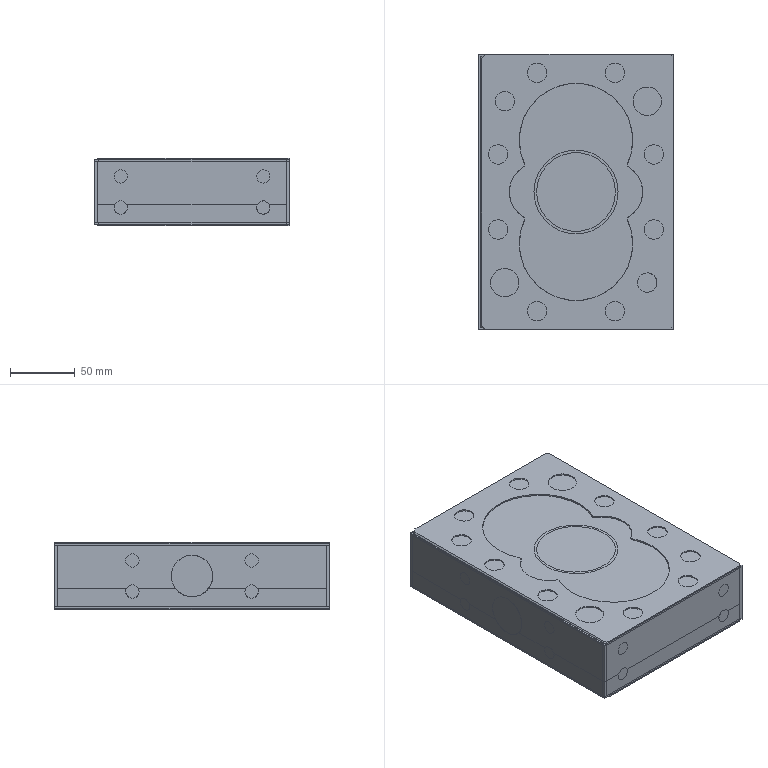NC program | NX | posted with a generic post | part box 150.2 x 212.2 x 52.4 mm
Whole program:
N10 G17 G21 G94 G90
(G81点孔_2 , TOOL : D6点孔钻_1)
N12 T01 M6
N14 /M1
N16 G54
N18 G17 G0 G90 X-46. Y-12. S2500 M3
N20 G43 Z20. H1
N22 G94 G81 G98 Z-1.5 F120. R1.5
N24 Y12.
N26 X0. Y0.
N28 X46. Y-12.
N30 Y12.
N32 G80
N34 G0 X46. Y12. Z20.
N36 M5
(G81点孔_3 , TOOL : Z3.3钻头)
N38 T03 M6
N40 /M1
N42 G54
N44 G17 G0 G90 X0. Y0. S500 M3
N46 G43 Z20. H3
N48 G94 G81 G98 Z-30. F20. R1.5
N50 G80
N52 G0 X0. Y0. Z20.
N54 M5
(孔铣开粗_3 , TOOL : D21R0.8圆鼻飞刀)
N56 T04 M6
N58 /M1
N60 G54
N62 G17 G0 G90 X0. Y0. S2000 M3
N64 G43 Z20. H4
N66 Z1.2
N68 G94 G1 Z0.2 F1200.
N70 G3 X-1.6 Y1.6 R1.6
N72 X-3.2 Y0. R1.6
N74 X-3.2 Y0. Z0. I3.2 J0. F1500.
N76 X-3.2 Y0. Z-0.2 I3.2 J0.
N78 X-3.2 Y0. Z-0.4 I3.2 J0.
N80 X-3.2 Y0. Z-0.6 I3.2 J0.
N82 X-3.2 Y0. Z-0.8 I3.2 J0.
N84 X-3.2 Y0. Z-1. I3.2 J0.
N86 X-3.2 Y0. Z-1.2 I3.2 J0.
N88 X-3.2 Y0. Z-1.4 I3.2 J0.
N90 X-3.2 Y0. Z-1.6 I3.2 J0.
N92 X-3.2 Y0. Z-1.8 I3.2 J0.
N94 X-3.2 Y0. Z-2. I3.2 J0.
N96 X-3.2 Y0. Z-2.2 I3.2 J0.
N98 X-3.2 Y0. Z-2.4 I3.2 J0.
N100 X-3.2 Y0. Z-2.6 I3.2 J0.
N102 X-3.2 Y0. Z-2.8 I3.2 J0.
N104 X-3.2 Y0. Z-3. I3.2 J0.
N106 X-3.2 Y0. Z-3.2 I3.2 J0.
N108 X-3.2 Y0. Z-3.4 I3.2 J0.
N110 X-3.2 Y0. Z-3.6 I3.2 J0.
N112 X-3.2 Y0. Z-3.8 I3.2 J0.
N114 X-3.2 Y0. Z-4. I3.2 J0.
N116 X-3.2 Y0. Z-4.2 I3.2 J0.
N118 X-3.2 Y0. Z-4.4 I3.2 J0.
N120 X-3.2 Y0. Z-4.6 I3.2 J0.
N122 X-3.2 Y0. Z-4.8 I3.2 J0.
N124 X-3.2 Y0. Z-5. I3.2 J0.
N126 X-3.2 Y0. Z-5.2 I3.2 J0.
N128 X-3.2 Y0. Z-5.4 I3.2 J0.
N130 X-3.2 Y0. Z-5.6 I3.2 J0.
N132 X-3.2 Y0. Z-5.8 I3.2 J0.
N134 X-3.2 Y0. Z-6. I3.2 J0.
N136 X-3.2 Y0. Z-6.2 I3.2 J0.
N138 X-3.2 Y0. Z-6.4 I3.2 J0.
N140 X-3.2 Y0. Z-6.6 I3.2 J0.
N142 X-3.2 Y0. Z-6.8 I3.2 J0.
N144 X-3.2 Y0. Z-7. I3.2 J0.
N146 X-3.2 Y0. Z-7.2 I3.2 J0.
N148 X-3.2 Y0. Z-7.4 I3.2 J0.
N150 X-3.2 Y0. Z-7.6 I3.2 J0.
N152 X-3.2 Y0. Z-7.8 I3.2 J0.
N154 X-3.2 Y0. Z-8. I3.2 J0.
N156 X-3.2 Y0. Z-8.2 I3.2 J0.
N158 X-3.2 Y0. Z-8.4 I3.2 J0.
N160 X-3.2 Y0. Z-8.6 I3.2 J0.
N162 X-3.2 Y0. Z-8.8 I3.2 J0.
N164 X-3.2 Y0. Z-9. I3.2 J0.
N166 X-3.2 Y0. Z-9.2 I3.2 J0.
N168 X-3.2 Y0. Z-9.4 I3.2 J0.
N170 X-3.2 Y0. Z-9.6 I3.2 J0.
N172 X-3.2 Y0. Z-9.8 I3.2 J0.
N174 X-3.2 Y0. Z-10. I3.2 J0.
N176 X-3.2 Y0. Z-10.2 I3.2 J0.
N178 X-3.2 Y0. Z-10.4 I3.2 J0.
N180 X-3.2 Y0. Z-10.6 I3.2 J0.
N182 X-3.2 Y0. Z-10.8 I3.2 J0.
N184 X-3.2 Y0. Z-11. I3.2 J0.
N186 X-3.2 Y0. Z-11.2 I3.2 J0.
N188 X-3.2 Y0. Z-11.4 I3.2 J0.
N190 X-3.2 Y0. Z-11.6 I3.2 J0.
N192 X-3.2 Y0. Z-11.8 I3.2 J0.
N194 X-3.2 Y0. Z-12. I3.2 J0.
N196 X-3.2 Y0. Z-12.2 I3.2 J0.
N198 X-3.2 Y0. Z-12.4 I3.2 J0.
N200 X-3.2 Y0. Z-12.6 I3.2 J0.
N202 X-3.2 Y0. Z-12.8 I3.2 J0.
N204 X-3.2 Y0. Z-13. I3.2 J0.
N206 X-3.2 Y0. Z-13.2 I3.2 J0.
N208 X-3.2 Y0. Z-13.4 I3.2 J0.
N210 X-3.2 Y0. Z-13.6 I3.2 J0.
N212 X-3.2 Y0. Z-13.8 I3.2 J0.
N214 X-3.2 Y0. Z-14. I3.2 J0.
N216 X-3.2 Y0. Z-14.2 I3.2 J0.
N218 X-3.2 Y0. Z-14.4 I3.2 J0.
N220 X-3.2 Y0. Z-14.6 I3.2 J0.
N222 X-3.2 Y0. Z-14.8 I3.2 J0.
N224 X-3.2 Y0. Z-15. I3.2 J0.
N226 X-3.2 Y0. Z-15.2 I3.2 J0.
N228 X-3.2 Y0. Z-15.4 I3.2 J0.
N230 X-3.2 Y0. Z-15.6 I3.2 J0.
N232 X-3.2 Y0. Z-15.8 I3.2 J0.
N234 X-3.2 Y0. Z-16. I3.2 J0.
N236 X-3.2 Y0. Z-16.2 I3.2 J0.
N238 X-3.2 Y0. Z-16.4 I3.2 J0.
N240 X-3.2 Y0. Z-16.6 I3.2 J0.
N242 X-3.2 Y0. Z-16.8 I3.2 J0.
N244 X-3.2 Y0. Z-17. I3.2 J0.
N246 X-3.2 Y0. Z-17.2 I3.2 J0.
N248 X-3.2 Y0. Z-17.4 I3.2 J0.
N250 X-3.2 Y0. Z-17.6 I3.2 J0.
N252 X-3.2 Y0. Z-17.8 I3.2 J0.
N254 X-3.2 Y0. Z-18. I3.2 J0.
N256 X-3.2 Y0. Z-18.2 I3.2 J0.
N258 X-3.2 Y0. Z-18.4 I3.2 J0.
N260 X-3.2 Y0. Z-18.6 I3.2 J0.
N262 X-3.2 Y0. Z-18.8 I3.2 J0.
N264 X-3.2 Y0. Z-19. I3.2 J0.
N266 X-3.2 Y0. Z-19.2 I3.2 J0.
N268 X-3.2 Y0. Z-19.4 I3.2 J0.
N270 X-3.2 Y0. Z-19.6 I3.2 J0.
N272 X-3.2 Y0. Z-19.8 I3.2 J0.
N274 X-3.2 Y0. Z-20. I3.2 J0.
N276 X-3.2 Y0. Z-20.2 I3.2 J0.
N278 X-3.2 Y0. Z-20.4 I3.2 J0.
N280 X-3.2 Y0. Z-20.6 I3.2 J0.
N282 X-3.2 Y0. Z-20.8 I3.2 J0.
N284 X-3.2 Y0. Z-21. I3.2 J0.
N286 X-3.2 Y0. Z-21.2 I3.2 J0.
N288 X-3.2 Y0. Z-21.4 I3.2 J0.
N290 X-3.2 Y0. Z-21.6 I3.2 J0.
N292 X-3.2 Y0. Z-21.8 I3.2 J0.
N294 X-3.2 Y0. Z-22. I3.2 J0.
N296 X-3.2 Y0. Z-22.2 I3.2 J0.
N298 X-3.2 Y0. Z-22.4 I3.2 J0.
N300 X-3.2 Y0. Z-22.6 I3.2 J0.
N302 X-3.2 Y0. Z-22.8 I3.2 J0.
N304 X-3.2 Y0. Z-23. I3.2 J0.
N306 X-3.2 Y0. Z-23.2 I3.2 J0.
N308 X-3.2 Y0. Z-23.4 I3.2 J0.
N310 X-3.2 Y0. Z-23.6 I3.2 J0.
N312 X-3.2 Y0. Z-23.8 I3.2 J0.
N314 X-3.2 Y0. Z-24. I3.2 J0.
N316 X-3.2 Y0. Z-24.2 I3.2 J0.
N318 X-3.2 Y0. Z-24.4 I3.2 J0.
N320 X-3.2 Y0. Z-24.6 I3.2 J0.
N322 X-3.2 Y0. Z-24.8 I3.2 J0.
N324 X-3.2 Y0. Z-25. I3.2 J0.
N326 X-3.2 Y0. Z-25.2 I3.2 J0.
N328 X-3.2 Y0. Z-25.4 I3.2 J0.
N330 X-3.2 Y0. Z-25.6 I3.2 J0.
N332 X-3.2 Y0. Z-25.8 I3.2 J0.
N334 X-3.2 Y0. Z-26. I3.2 J0.
N336 X-3.2 Y0. Z-26.2 I3.2 J0.
N338 X-3.2 Y0. Z-26.4 I3.2 J0.
N340 X-3.2 Y0. Z-26.6 I3.2 J0.
N342 X-3.2 Y0. Z-26.8 I3.2 J0.
N344 X-3.2 Y0. Z-27. I3.2 J0.
N346 X-3.2 Y0. Z-27.2 I3.2 J0.
N348 X-3.2 Y0. Z-27.4 I3.2 J0.
N350 X-3.2 Y0. Z-27.6 I3.2 J0.
N352 X-3.2 Y0. Z-27.8 I3.2 J0.
N354 X-3.2 Y0. Z-28. I3.2 J0.
N356 X-3.2 Y0. Z-28.2 I3.2 J0.
N358 X-3.2 Y0. Z-28.4 I3.2 J0.
N360 X-3.2 Y0. Z-28.6 I3.2 J0.
N362 X-3.2 Y0. Z-28.8 I3.2 J0.
N364 X-3.2 Y0. Z-29. I3.2 J0.
N366 X-3.2 Y0. Z-29.2 I3.2 J0.
N368 X-3.2 Y0. Z-29.4 I3.2 J0.
N370 X-3.2 Y0. Z-29.6 I3.2 J0.
N372 X-3.2 Y0. Z-29.8 I3.2 J0.
N374 X-3.2 Y0. Z-30. I3.2 J0.
N376 X-3.2 Y0. Z-30.2 I3.2 J0.
N378 X-3.2 Y0. Z-30.4 I3.2 J0.
N380 X-3.2 Y0. Z-30.6 I3.2 J0.
N382 X-3.2 Y0. Z-30.8 I3.2 J0.
N384 X-3.2 Y0. Z-31. I3.2 J0.
N386 X-3.2 Y0. Z-31.2 I3.2 J0.
N388 X-3.2 Y0. Z-31.4 I3.2 J0.
N390 X-3.2 Y0. Z-31.6 I3.2 J0.
N392 X-3.2 Y0. Z-31.8 I3.2 J0.
N394 X-3.2 Y0. Z-32. I3.2 J0.
N396 X-3.2 Y0. Z-32.2 I3.2 J0.
N398 X-3.2 Y0. Z-32.4 I3.2 J0.
N400 X-3.2 Y0. Z-32.6 I3.2 J0.
N402 X-3.2 Y0. Z-32.8 I3.2 J0.
N404 X-3.2 Y0. Z-33. I3.2 J0.
N406 X-3.2 Y0. Z-33.2 I3.2 J0.
N408 X-3.2 Y0. Z-33.4 I3.2 J0.
N410 X-3.2 Y0. Z-33.6 I3.2 J0.
N412 X-3.2 Y0. Z-33.8 I3.2 J0.
N414 X-3.2 Y0. Z-34. I3.2 J0.
N416 X-3.2 Y0. Z-34.2 I3.2 J0.
N418 X-3.2 Y0. Z-34.4 I3.2 J0.
N420 X-3.2 Y0. Z-34.6 I3.2 J0.
N422 X-3.2 Y0. Z-34.8 I3.2 J0.
N424 X-3.2 Y0. Z-35. I3.2 J0.
N426 X0. Y-3.2 R3.2
N428 X-3.2 Y0. R-3.2
N430 X-1.6 Y-1.6 R1.6
N432 X0. Y0. R1.6
N434 G0 Z20.
N436 M5
(G81点孔_7 , TOOL : D16平底刀)
N438 T02 M6
N440 /M1
N442 G54
N444 G17 G0 G90 X0. Y0. S500 M3
N446 G43 Z20. H2
N448 G94 G85 G98 Z-31.781 F50. R1.5
N450 G80
N452 G0 X0. Y0. Z20.
N454 M5
(G83钻孔_1 , TOOL : Z1.6钻头)
N456 T18 M6
N458 /M1
N460 G54
N462 G17 G0 G90 X46. Y12. S800 M3
N464 G43 Z20. H18
N466 G94 G83 G98 Z-20. F42. Q1. R1.5
N468 X-46. Y-12.
N470 X46.
N472 X-46. Y12.
N474 G80
N476 G0 X-46. Y12. Z20.
N478 M5
(孔铣开粗_2 , TOOL : D10平底刀)
N480 T15 M6
N482 /M1
N484 G54
N486 G17 G0 G90 X-46. Y12. S1700 M3
N488 G43 Z20. H15
N490 Z1.2
N492 G94 G1 Z0.2 F160.
N494 G3 X-46.075 Y12.075 R0.075
N496 X-46.15 Y12. R0.075
N498 X-46.15 Y12. Z0. I0.15 J0. F200.
N500 X-46.15 Y12. Z-0.2 I0.15 J0.
N502 X-46.15 Y12. Z-0.4 I0.15 J0.
N504 X-46.15 Y12. Z-0.6 I0.15 J0.
N506 X-46.15 Y12. Z-0.8 I0.15 J0.
N508 X-46.15 Y12. Z-1. I0.15 J0.
N510 X-46.15 Y12. Z-1.2 I0.15 J0.
N512 X-46.15 Y12. Z-1.4 I0.15 J0.
N514 X-46.15 Y12. Z-1.6 I0.15 J0.
N516 X-46.15 Y12. Z-1.8 I0.15 J0.
N518 X-46.15 Y12. Z-2. I0.15 J0.
N520 X-46.15 Y12. Z-2.2 I0.15 J0.
N522 X-46.15 Y12. Z-2.4 I0.15 J0.
N524 X-46.15 Y12. Z-2.6 I0.15 J0.
N526 X-46.15 Y12. Z-2.8 I0.15 J0.
N528 X-46.15 Y12. Z-3. I0.15 J0.
N530 X-46.15 Y12. Z-3.2 I0.15 J0.
N532 X-46.15 Y12. Z-3.4 I0.15 J0.
N534 X-46.15 Y12. Z-3.6 I0.15 J0.
N536 X-46.15 Y12. Z-3.8 I0.15 J0.
N538 X-46.15 Y12. Z-4. I0.15 J0.
N540 X-46.15 Y12. Z-4.2 I0.15 J0.
N542 X-46.15 Y12. Z-4.4 I0.15 J0.
N544 X-46.15 Y12. Z-4.6 I0.15 J0.
N546 X-46.15 Y12. Z-4.8 I0.15 J0.
N548 X-46.15 Y12. Z-5. I0.15 J0.
N550 X-46.15 Y12. Z-5.2 I0.15 J0.
N552 X-46.15 Y12. Z-5.4 I0.15 J0.
N554 X-46.15 Y12. Z-5.6 I0.15 J0.
N556 X-46.15 Y12. Z-5.8 I0.15 J0.
N558 X-46.15 Y12. Z-6. I0.15 J0.
N560 X-46.15 Y12. Z-6.2 I0.15 J0.
N562 X-46.15 Y12. Z-6.4 I0.15 J0.
N564 X-46.15 Y12. Z-6.6 I0.15 J0.
N566 X-46.15 Y12. Z-6.8 I0.15 J0.
N568 X-46.15 Y12. Z-7. I0.15 J0.
N570 X-46.15 Y12. Z-7.2 I0.15 J0.
N572 X-46.15 Y12. Z-7.4 I0.15 J0.
N574 X-46.15 Y12. Z-7.6 I0.15 J0.
N576 X-46.15 Y12. Z-7.8 I0.15 J0.
N578 X-46.15 Y12. Z-8. I0.15 J0.
N580 X-46.15 Y12. Z-8.2 I0.15 J0.
N582 X-46.15 Y12. Z-8.4 I0.15 J0.
N584 X-46.15 Y12. Z-8.6 I0.15 J0.
N586 X-46.15 Y12. Z-8.8 I0.15 J0.
N588 X-46.15 Y12. Z-9. I0.15 J0.
N590 X-46.15 Y12. Z-9.2 I0.15 J0.
N592 X-46.15 Y12. Z-9.4 I0.15 J0.
N594 X-46.15 Y12. Z-9.6 I0.15 J0.
N596 X-46.15 Y12. Z-9.8 I0.15 J0.
N598 X-46.15 Y12. Z-10. I0.15 J0.
N600 X-46.15 Y12. Z-10.2 I0.15 J0.
N602 X-46.15 Y12. Z-10.4 I0.15 J0.
N604 X-46.15 Y12. Z-10.6 I0.15 J0.
N606 X-46.15 Y12. Z-10.8 I0.15 J0.
N608 X-46.15 Y12. Z-11. I0.15 J0.
N610 X-46.15 Y12. Z-11.2 I0.15 J0.
N612 X-46.15 Y12. Z-11.4 I0.15 J0.
N614 X-46.15 Y12. Z-11.6 I0.15 J0.
N616 X-46.15 Y12. Z-11.8 I0.15 J0.
N618 X-46.15 Y12. Z-12. I0.15 J0.
N620 X-46.15 Y12. Z-12.2 I0.15 J0.
N622 X-46.15 Y12. Z-12.4 I0.15 J0.
N624 X-46.15 Y12. Z-12.6 I0.15 J0.
N626 X-46.15 Y12. Z-12.8 I0.15 J0.
N628 X-46.15 Y12. Z-13. I0.15 J0.
N630 X-46.15 Y12. Z-13.2 I0.15 J0.
N632 X-46.15 Y12. Z-13.4 I0.15 J0.
N634 X-46.15 Y12. Z-13.6 I0.15 J0.
N636 X-46.15 Y12. Z-13.8 I0.15 J0.
N638 X-46.15 Y12. Z-14. I0.15 J0.
N640 X-46.15 Y12. Z-14.2 I0.15 J0.
N642 X-46.15 Y12. Z-14.4 I0.15 J0.
N644 X-46.15 Y12. Z-14.6 I0.15 J0.
N646 X-46.15 Y12. Z-14.8 I0.15 J0.
N648 X-46.15 Y12. Z-15. I0.15 J0.
N650 X-46.15 Y12. Z-15.2 I0.15 J0.
N652 X-46.15 Y12. Z-15.4 I0.15 J0.
N654 X-46.15 Y12. Z-15.6 I0.15 J0.
N656 X-46.15 Y12. Z-15.8 I0.15 J0.
N658 X-46.15 Y12. Z-16. I0.15 J0.
N660 X-46.15 Y12. Z-16.2 I0.15 J0.
N662 X-46.15 Y12. Z-16.4 I0.15 J0.
N664 X-46.15 Y12. Z-16.6 I0.15 J0.
N666 X-46.15 Y12. Z-16.8 I0.15 J0.
N668 X-46.15 Y12. Z-17. I0.15 J0.
N670 X-46.15 Y12. Z-17.2 I0.15 J0.
N672 X-46.15 Y12. Z-17.4 I0.15 J0.
N674 X-46.15 Y12. Z-17.6 I0.15 J0.
N676 X-46.15 Y12. Z-17.8 I0.15 J0.
N678 X-46.15 Y12. Z-18. I0.15 J0.
N680 X-46.15 Y12. Z-18.2 I0.15 J0.
N682 X-46.15 Y12. Z-18.4 I0.15 J0.
N684 X-46.15 Y12. Z-18.6 I0.15 J0.
N686 X-46.15 Y12. Z-18.8 I0.15 J0.
N688 X-46.15 Y12. Z-19. I0.15 J0.
N690 X-46.15 Y12. Z-19.2 I0.15 J0.
N692 X-46.15 Y12. Z-19.4 I0.15 J0.
N694 X-46.15 Y12. Z-19.6 I0.15 J0.
N696 X-46.15 Y12. Z-19.8 I0.15 J0.
N698 X-46.15 Y12. Z-20. I0.15 J0.
N700 X-46.15 Y12. Z-20.2 I0.15 J0.
N702 X-46.15 Y12. Z-20.4 I0.15 J0.
N704 X-46.15 Y12. Z-20.6 I0.15 J0.
N706 X-46.15 Y12. Z-20.8 I0.15 J0.
N708 X-46.15 Y12. Z-21. I0.15 J0.
N710 X-46.15 Y12. Z-21.2 I0.15 J0.
N712 X-46.15 Y12. Z-21.4 I0.15 J0.
N714 X-46.15 Y12. Z-21.6 I0.15 J0.
N716 X-46.15 Y12. Z-21.8 I0.15 J0.
N718 X-46.15 Y12. Z-22. I0.15 J0.
N720 X-46.15 Y12. Z-22.2 I0.15 J0.
N722 X-46.15 Y12. Z-22.4 I0.15 J0.
N724 X-46.15 Y12. Z-22.6 I0.15 J0.
N726 X-46.15 Y12. Z-22.8 I0.15 J0.
N728 X-46.15 Y12. Z-23. I0.15 J0.
N730 X-46. Y11.85 R0.15
N732 X-46.15 Y12. R-0.15
N734 X-46.075 Y11.925 R0.075
N736 X-46. Y12. R0.075
N738 G0 Z20.
N740 X46.
N742 Z1.2
N744 G1 Z0.2 F160.
N746 G3 X45.925 Y12.075 R0.075
N748 X45.85 Y12. R0.075
N750 X45.85 Y12. Z0. I0.15 J0. F200.
N752 X45.85 Y12. Z-0.2 I0.15 J0.
N754 X45.85 Y12. Z-0.4 I0.15 J0.
N756 X45.85 Y12. Z-0.6 I0.15 J0.
N758 X45.85 Y12. Z-0.8 I0.15 J0.
N760 X45.85 Y12. Z-1. I0.15 J0.
N762 X45.85 Y12. Z-1.2 I0.15 J0.
N764 X45.85 Y12. Z-1.4 I0.15 J0.
N766 X45.85 Y12. Z-1.6 I0.15 J0.
N768 X45.85 Y12. Z-1.8 I0.15 J0.
N770 X45.85 Y12. Z-2. I0.15 J0.
N772 X45.85 Y12. Z-2.2 I0.15 J0.
N774 X45.85 Y12. Z-2.4 I0.15 J0.
N776 X45.85 Y12. Z-2.6 I0.15 J0.
N778 X45.85 Y12. Z-2.8 I0.15 J0.
N780 X45.85 Y12. Z-3. I0.15 J0.
N782 X45.85 Y12. Z-3.2 I0.15 J0.
N784 X45.85 Y12. Z-3.4 I0.15 J0.
N786 X45.85 Y12. Z-3.6 I0.15 J0.
N788 X45.85 Y12. Z-3.8 I0.15 J0.
N790 X45.85 Y12. Z-4. I0.15 J0.
N792 X45.85 Y12. Z-4.2 I0.15 J0.
N794 X45.85 Y12. Z-4.4 I0.15 J0.
N796 X45.85 Y12. Z-4.6 I0.15 J0.
N798 X45.85 Y12. Z-4.8 I0.15 J0.
N800 X45.85 Y12. Z-5. I0.15 J0.
N802 X45.85 Y12. Z-5.2 I0.15 J0.
N804 X45.85 Y12. Z-5.4 I0.15 J0.
N806 X45.85 Y12. Z-5.6 I0.15 J0.
N808 X45.85 Y12. Z-5.8 I0.15 J0.
N810 X45.85 Y12. Z-6. I0.15 J0.
N812 X45.85 Y12. Z-6.2 I0.15 J0.
N814 X45.85 Y12. Z-6.4 I0.15 J0.
N816 X45.85 Y12. Z-6.6 I0.15 J0.
N818 X45.85 Y12. Z-6.8 I0.15 J0.
N820 X45.85 Y12. Z-7. I0.15 J0.
N822 X45.85 Y12. Z-7.2 I0.15 J0.
N824 X45.85 Y12. Z-7.4 I0.15 J0.
N826 X45.85 Y12. Z-7.6 I0.15 J0.
N828 X45.85 Y12. Z-7.8 I0.15 J0.
N830 X45.85 Y12. Z-8. I0.15 J0.
N832 X45.85 Y12. Z-8.2 I0.15 J0.
N834 X45.85 Y12. Z-8.4 I0.15 J0.
N836 X45.85 Y12. Z-8.6 I0.15 J0.
N838 X45.85 Y12. Z-8.8 I0.15 J0.
N840 X45.85 Y12. Z-9. I0.15 J0.
N842 X45.85 Y12. Z-9.2 I0.15 J0.
N844 X45.85 Y12. Z-9.4 I0.15 J0.
N846 X45.85 Y12. Z-9.6 I0.15 J0.
N848 X45.85 Y12. Z-9.8 I0.15 J0.
N850 X45.85 Y12. Z-10. I0.15 J0.
N852 X45.85 Y12. Z-10.2 I0.15 J0.
N854 X45.85 Y12. Z-10.4 I0.15 J0.
N856 X45.85 Y12. Z-10.6 I0.15 J0.
N858 X45.85 Y12. Z-10.8 I0.15 J0.
N860 X45.85 Y12. Z-11. I0.15 J0.
N862 X45.85 Y12. Z-11.2 I0.15 J0.
N864 X45.85 Y12. Z-11.4 I0.15 J0.
N866 X45.85 Y12. Z-11.6 I0.15 J0.
N868 X45.85 Y12. Z-11.8 I0.15 J0.
N870 X45.85 Y12. Z-12. I0.15 J0.
N872 X45.85 Y12. Z-12.2 I0.15 J0.
N874 X45.85 Y12. Z-12.4 I0.15 J0.
N876 X45.85 Y12. Z-12.6 I0.15 J0.
N878 X45.85 Y12. Z-12.8 I0.15 J0.
N880 X45.85 Y12. Z-13. I0.15 J0.
N882 X45.85 Y12. Z-13.2 I0.15 J0.
N884 X45.85 Y12. Z-13.4 I0.15 J0.
N886 X45.85 Y12. Z-13.6 I0.15 J0.
N888 X45.85 Y12. Z-13.8 I0.15 J0.
N890 X45.85 Y12. Z-14. I0.15 J0.
N892 X45.85 Y12. Z-14.2 I0.15 J0.
N894 X45.85 Y12. Z-14.4 I0.15 J0.
N896 X45.85 Y12. Z-14.6 I0.15 J0.
N898 X45.85 Y12. Z-14.8 I0.15 J0.
N900 X45.85 Y12. Z-15. I0.15 J0.
N902 X45.85 Y12. Z-15.2 I0.15 J0.
N904 X45.85 Y12. Z-15.4 I0.15 J0.
N906 X45.85 Y12. Z-15.6 I0.15 J0.
N908 X45.85 Y12. Z-15.8 I0.15 J0.
N910 X45.85 Y12. Z-16. I0.15 J0.
N912 X45.85 Y12. Z-16.2 I0.15 J0.
N914 X45.85 Y12. Z-16.4 I0.15 J0.
N916 X45.85 Y12. Z-16.6 I0.15 J0.
N918 X45.85 Y12. Z-16.8 I0.15 J0.
N920 X45.85 Y12. Z-17. I0.15 J0.
N922 X45.85 Y12. Z-17.2 I0.15 J0.
N924 X45.85 Y12. Z-17.4 I0.15 J0.
N926 X45.85 Y12. Z-17.6 I0.15 J0.
N928 X45.85 Y12. Z-17.8 I0.15 J0.
N930 X45.85 Y12. Z-18. I0.15 J0.
N932 X45.85 Y12. Z-18.2 I0.15 J0.
N934 X45.85 Y12. Z-18.4 I0.15 J0.
N936 X45.85 Y12. Z-18.6 I0.15 J0.
N938 X45.85 Y12. Z-18.8 I0.15 J0.
N940 X45.85 Y12. Z-19. I0.15 J0.
N942 X45.85 Y12. Z-19.2 I0.15 J0.
N944 X45.85 Y12. Z-19.4 I0.15 J0.
N946 X45.85 Y12. Z-19.6 I0.15 J0.
N948 X45.85 Y12. Z-19.8 I0.15 J0.
N950 X45.85 Y12. Z-20. I0.15 J0.
N952 X45.85 Y12. Z-20.2 I0.15 J0.
N954 X45.85 Y12. Z-20.4 I0.15 J0.
N956 X45.85 Y12. Z-20.6 I0.15 J0.
N958 X45.85 Y12. Z-20.8 I0.15 J0.
N960 X45.85 Y12. Z-21. I0.15 J0.
N962 X45.85 Y12. Z-21.2 I0.15 J0.
N964 X45.85 Y12. Z-21.4 I0.15 J0.
N966 X45.85 Y12. Z-21.6 I0.15 J0.
N968 X45.85 Y12. Z-21.8 I0.15 J0.
N970 X45.85 Y12. Z-22. I0.15 J0.
N972 X45.85 Y12. Z-22.2 I0.15 J0.
N974 X45.85 Y12. Z-22.4 I0.15 J0.
N976 X45.85 Y12. Z-22.6 I0.15 J0.
N978 X45.85 Y12. Z-22.8 I0.15 J0.
N980 X45.85 Y12. Z-23. I0.15 J0.
N982 X46. Y11.85 R0.15
N984 X45.85 Y12. R-0.15
N986 X45.925 Y11.925 R0.075
N988 X46. Y12. R0.075
N990 G0 Z20.
N992 Y-12.
N994 Z1.2
N996 G1 Z0.2 F160.
N998 G3 X45.925 Y-11.925 R0.075
N1000 X45.85 Y-12. R0.075
N1002 X45.85 Y-12. Z0. I0.15 J0. F200.
N1004 X45.85 Y-12. Z-0.2 I0.15 J0.
N1006 X45.85 Y-12. Z-0.4 I0.15 J0.
N1008 X45.85 Y-12. Z-0.6 I0.15 J0.
N1010 X45.85 Y-12. Z-0.8 I0.15 J0.
N1012 X45.85 Y-12. Z-1. I0.15 J0.
N1014 X45.85 Y-12. Z-1.2 I0.15 J0.
N1016 X45.85 Y-12. Z-1.4 I0.15 J0.
N1018 X45.85 Y-12. Z-1.6 I0.15 J0.
N1020 X45.85 Y-12. Z-1.8 I0.15 J0.
N1022 X45.85 Y-12. Z-2. I0.15 J0.
N1024 X45.85 Y-12. Z-2.2 I0.15 J0.
N1026 X45.85 Y-12. Z-2.4 I0.15 J0.
N1028 X45.85 Y-12. Z-2.6 I0.15 J0.
N1030 X45.85 Y-12. Z-2.8 I0.15 J0.
N1032 X45.85 Y-12. Z-3. I0.15 J0.
N1034 X45.85 Y-12. Z-3.2 I0.15 J0.
N1036 X45.85 Y-12. Z-3.4 I0.15 J0.
N1038 X45.85 Y-12. Z-3.6 I0.15 J0.
N1040 X45.85 Y-12. Z-3.8 I0.15 J0.
N1042 X45.85 Y-12. Z-4. I0.15 J0.
N1044 X45.85 Y-12. Z-4.2 I0.15 J0.
N1046 X45.85 Y-12. Z-4.4 I0.15 J0.
N1048 X45.85 Y-12. Z-4.6 I0.15 J0.
N1050 X45.85 Y-12. Z-4.8 I0.15 J0.
N1052 X45.85 Y-12. Z-5. I0.15 J0.
N1054 X45.85 Y-12. Z-5.2 I0.15 J0.
N1056 X45.85 Y-12. Z-5.4 I0.15 J0.
N1058 X45.85 Y-12. Z-5.6 I0.15 J0.
N1060 X45.85 Y-12. Z-5.8 I0.15 J0.
N1062 X45.85 Y-12. Z-6. I0.15 J0.
N1064 X45.85 Y-12. Z-6.2 I0.15 J0.
N1066 X45.85 Y-12. Z-6.4 I0.15 J0.
N1068 X45.85 Y-12. Z-6.6 I0.15 J0.
N1070 X45.85 Y-12. Z-6.8 I0.15 J0.
N1072 X45.85 Y-12. Z-7. I0.15 J0.
N1074 X45.85 Y-12. Z-7.2 I0.15 J0.
N1076 X45.85 Y-12. Z-7.4 I0.15 J0.
N1078 X45.85 Y-12. Z-7.6 I0.15 J0.
N1080 X45.85 Y-12. Z-7.8 I0.15 J0.
N1082 X45.85 Y-12. Z-8. I0.15 J0.
N1084 X45.85 Y-12. Z-8.2 I0.15 J0.
N1086 X45.85 Y-12. Z-8.4 I0.15 J0.
N1088 X45.85 Y-12. Z-8.6 I0.15 J0.
N1090 X45.85 Y-12. Z-8.8 I0.15 J0.
N1092 X45.85 Y-12. Z-9. I0.15 J0.
N1094 X45.85 Y-12. Z-9.2 I0.15 J0.
N1096 X45.85 Y-12. Z-9.4 I0.15 J0.
N1098 X45.85 Y-12. Z-9.6 I0.15 J0.
N1100 X45.85 Y-12. Z-9.8 I0.15 J0.
N1102 X45.85 Y-12. Z-10. I0.15 J0.
N1104 X45.85 Y-12. Z-10.2 I0.15 J0.
N1106 X45.85 Y-12. Z-10.4 I0.15 J0.
N1108 X45.85 Y-12. Z-10.6 I0.15 J0.
N1110 X45.85 Y-12. Z-10.8 I0.15 J0.
N1112 X45.85 Y-12. Z-11. I0.15 J0.
N1114 X45.85 Y-12. Z-11.2 I0.15 J0.
N1116 X45.85 Y-12. Z-11.4 I0.15 J0.
N1118 X45.85 Y-12. Z-11.6 I0.15 J0.
N1120 X45.85 Y-12. Z-11.8 I0.15 J0.
N1122 X45.85 Y-12. Z-12. I0.15 J0.
N1124 X45.85 Y-12. Z-12.2 I0.15 J0.
N1126 X45.85 Y-12. Z-12.4 I0.15 J0.
N1128 X45.85 Y-12. Z-12.6 I0.15 J0.
N1130 X45.85 Y-12. Z-12.8 I0.15 J0.
N1132 X45.85 Y-12. Z-13. I0.15 J0.
N1134 X45.85 Y-12. Z-13.2 I0.15 J0.
N1136 X45.85 Y-12. Z-13.4 I0.15 J0.
N1138 X45.85 Y-12. Z-13.6 I0.15 J0.
N1140 X45.85 Y-12. Z-13.8 I0.15 J0.
N1142 X45.85 Y-12. Z-14. I0.15 J0.
N1144 X45.85 Y-12. Z-14.2 I0.15 J0.
N1146 X45.85 Y-12. Z-14.4 I0.15 J0.
N1148 X45.85 Y-12. Z-14.6 I0.15 J0.
N1150 X45.85 Y-12. Z-14.8 I0.15 J0.
N1152 X45.85 Y-12. Z-15. I0.15 J0.
N1154 X45.85 Y-12. Z-15.2 I0.15 J0.
N1156 X45.85 Y-12. Z-15.4 I0.15 J0.
N1158 X45.85 Y-12. Z-15.6 I0.15 J0.
N1160 X45.85 Y-12. Z-15.8 I0.15 J0.
N1162 X45.85 Y-12. Z-16. I0.15 J0.
N1164 X45.85 Y-12. Z-16.2 I0.15 J0.
N1166 X45.85 Y-12. Z-16.4 I0.15 J0.
N1168 X45.85 Y-12. Z-16.6 I0.15 J0.
N1170 X45.85 Y-12. Z-16.8 I0.15 J0.
N1172 X45.85 Y-12. Z-17. I0.15 J0.
N1174 X45.85 Y-12. Z-17.2 I0.15 J0.
N1176 X45.85 Y-12. Z-17.4 I0.15 J0.
N1178 X45.85 Y-12. Z-17.6 I0.15 J0.
N1180 X45.85 Y-12. Z-17.8 I0.15 J0.
N1182 X45.85 Y-12. Z-18. I0.15 J0.
N1184 X45.85 Y-12. Z-18.2 I0.15 J0.
N1186 X45.85 Y-12. Z-18.4 I0.15 J0.
N1188 X45.85 Y-12. Z-18.6 I0.15 J0.
N1190 X45.85 Y-12. Z-18.8 I0.15 J0.
N1192 X45.85 Y-12. Z-19. I0.15 J0.
N1194 X45.85 Y-12. Z-19.2 I0.15 J0.
N1196 X45.85 Y-12. Z-19.4 I0.15 J0.
N1198 X45.85 Y-12. Z-19.6 I0.15 J0.
N1200 X45.85 Y-12. Z-19.8 I0.15 J0.
N1202 X45.85 Y-12. Z-20. I0.15 J0.
N1204 X45.85 Y-12. Z-20.2 I0.15 J0.
N1206 X45.85 Y-12. Z-20.4 I0.15 J0.
N1208 X45.85 Y-12. Z-20.6 I0.15 J0.
N1210 X45.85 Y-12. Z-20.8 I0.15 J0.
N1212 X45.85 Y-12. Z-21. I0.15 J0.
N1214 X45.85 Y-12. Z-21.2 I0.15 J0.
N1216 X45.85 Y-12. Z-21.4 I0.15 J0.
N1218 X45.85 Y-12. Z-21.6 I0.15 J0.
N1220 X45.85 Y-12. Z-21.8 I0.15 J0.
N1222 X45.85 Y-12. Z-22. I0.15 J0.
N1224 X45.85 Y-12. Z-22.2 I0.15 J0.
N1226 X45.85 Y-12. Z-22.4 I0.15 J0.
N1228 X45.85 Y-12. Z-22.6 I0.15 J0.
N1230 X45.85 Y-12. Z-22.8 I0.15 J0.
N1232 X45.85 Y-12. Z-23. I0.15 J0.
N1234 X46. Y-12.15 R0.15
N1236 X45.85 Y-12. R-0.15
N1238 X45.925 Y-12.075 R0.075
N1240 X46. Y-12. R0.075
N1242 G0 Z20.
N1244 X-46.
N1246 Z1.2
N1248 G1 Z0.2 F160.
N1250 G3 X-46.075 Y-11.925 R0.075
N1252 X-46.15 Y-12. R0.075
N1254 X-46.15 Y-12. Z0. I0.15 J0. F200.
N1256 X-46.15 Y-12. Z-0.2 I0.15 J0.
N1258 X-46.15 Y-12. Z-0.4 I0.15 J0.
N1260 X-46.15 Y-12. Z-0.6 I0.15 J0.
N1262 X-46.15 Y-12. Z-0.8 I0.15 J0.
N1264 X-46.15 Y-12. Z-1. I0.15 J0.
N1266 X-46.15 Y-12. Z-1.2 I0.15 J0.
N1268 X-46.15 Y-12. Z-1.4 I0.15 J0.
N1270 X-46.15 Y-12. Z-1.6 I0.15 J0.
N1272 X-46.15 Y-12. Z-1.8 I0.15 J0.
N1274 X-46.15 Y-12. Z-2. I0.15 J0.
N1276 X-46.15 Y-12. Z-2.2 I0.15 J0.
N1278 X-46.15 Y-12. Z-2.4 I0.15 J0.
N1280 X-46.15 Y-12. Z-2.6 I0.15 J0.
N1282 X-46.15 Y-12. Z-2.8 I0.15 J0.
N1284 X-46.15 Y-12. Z-3. I0.15 J0.
N1286 X-46.15 Y-12. Z-3.2 I0.15 J0.
N1288 X-46.15 Y-12. Z-3.4 I0.15 J0.
N1290 X-46.15 Y-12. Z-3.6 I0.15 J0.
N1292 X-46.15 Y-12. Z-3.8 I0.15 J0.
N1294 X-46.15 Y-12. Z-4. I0.15 J0.
N1296 X-46.15 Y-12. Z-4.2 I0.15 J0.
N1298 X-46.15 Y-12. Z-4.4 I0.15 J0.
N1300 X-46.15 Y-12. Z-4.6 I0.15 J0.
N1302 X-46.15 Y-12. Z-4.8 I0.15 J0.
N1304 X-46.15 Y-12. Z-5. I0.15 J0.
N1306 X-46.15 Y-12. Z-5.2 I0.15 J0.
N1308 X-46.15 Y-12. Z-5.4 I0.15 J0.
N1310 X-46.15 Y-12. Z-5.6 I0.15 J0.
N1312 X-46.15 Y-12. Z-5.8 I0.15 J0.
N1314 X-46.15 Y-12. Z-6. I0.15 J0.
N1316 X-46.15 Y-12. Z-6.2 I0.15 J0.
N1318 X-46.15 Y-12. Z-6.4 I0.15 J0.
N1320 X-46.15 Y-12. Z-6.6 I0.15 J0.
N1322 X-46.15 Y-12. Z-6.8 I0.15 J0.
N1324 X-46.15 Y-12. Z-7. I0.15 J0.
N1326 X-46.15 Y-12. Z-7.2 I0.15 J0.
N1328 X-46.15 Y-12. Z-7.4 I0.15 J0.
N1330 X-46.15 Y-12. Z-7.6 I0.15 J0.
N1332 X-46.15 Y-12. Z-7.8 I0.15 J0.
N1334 X-46.15 Y-12. Z-8. I0.15 J0.
N1336 X-46.15 Y-12. Z-8.2 I0.15 J0.
N1338 X-46.15 Y-12. Z-8.4 I0.15 J0.
N1340 X-46.15 Y-12. Z-8.6 I0.15 J0.
N1342 X-46.15 Y-12. Z-8.8 I0.15 J0.
N1344 X-46.15 Y-12. Z-9. I0.15 J0.
N1346 X-46.15 Y-12. Z-9.2 I0.15 J0.
N1348 X-46.15 Y-12. Z-9.4 I0.15 J0.
N1350 X-46.15 Y-12. Z-9.6 I0.15 J0.
N1352 X-46.15 Y-12. Z-9.8 I0.15 J0.
N1354 X-46.15 Y-12. Z-10. I0.15 J0.
N1356 X-46.15 Y-12. Z-10.2 I0.15 J0.
N1358 X-46.15 Y-12. Z-10.4 I0.15 J0.
N1360 X-46.15 Y-12. Z-10.6 I0.15 J0.
N1362 X-46.15 Y-12. Z-10.8 I0.15 J0.
N1364 X-46.15 Y-12. Z-11. I0.15 J0.
N1366 X-46.15 Y-12. Z-11.2 I0.15 J0.
N1368 X-46.15 Y-12. Z-11.4 I0.15 J0.
N1370 X-46.15 Y-12. Z-11.6 I0.15 J0.
N1372 X-46.15 Y-12. Z-11.8 I0.15 J0.
N1374 X-46.15 Y-12. Z-12. I0.15 J0.
N1376 X-46.15 Y-12. Z-12.2 I0.15 J0.
N1378 X-46.15 Y-12. Z-12.4 I0.15 J0.
N1380 X-46.15 Y-12. Z-12.6 I0.15 J0.
N1382 X-46.15 Y-12. Z-12.8 I0.15 J0.
N1384 X-46.15 Y-12. Z-13. I0.15 J0.
N1386 X-46.15 Y-12. Z-13.2 I0.15 J0.
N1388 X-46.15 Y-12. Z-13.4 I0.15 J0.
N1390 X-46.15 Y-12. Z-13.6 I0.15 J0.
N1392 X-46.15 Y-12. Z-13.8 I0.15 J0.
N1394 X-46.15 Y-12. Z-14. I0.15 J0.
N1396 X-46.15 Y-12. Z-14.2 I0.15 J0.
N1398 X-46.15 Y-12. Z-14.4 I0.15 J0.
N1400 X-46.15 Y-12. Z-14.6 I0.15 J0.
N1402 X-46.15 Y-12. Z-14.8 I0.15 J0.
N1404 X-46.15 Y-12. Z-15. I0.15 J0.
N1406 X-46.15 Y-12. Z-15.2 I0.15 J0.
N1408 X-46.15 Y-12. Z-15.4 I0.15 J0.
N1410 X-46.15 Y-12. Z-15.6 I0.15 J0.
N1412 X-46.15 Y-12. Z-15.8 I0.15 J0.
N1414 X-46.15 Y-12. Z-16. I0.15 J0.
N1416 X-46.15 Y-12. Z-16.2 I0.15 J0.
N1418 X-46.15 Y-12. Z-16.4 I0.15 J0.
N1420 X-46.15 Y-12. Z-16.6 I0.15 J0.
N1422 X-46.15 Y-12. Z-16.8 I0.15 J0.
N1424 X-46.15 Y-12. Z-17. I0.15 J0.
N1426 X-46.15 Y-12. Z-17.2 I0.15 J0.
N1428 X-46.15 Y-12. Z-17.4 I0.15 J0.
N1430 X-46.15 Y-12. Z-17.6 I0.15 J0.
N1432 X-46.15 Y-12. Z-17.8 I0.15 J0.
N1434 X-46.15 Y-12. Z-18. I0.15 J0.
N1436 X-46.15 Y-12. Z-18.2 I0.15 J0.
N1438 X-46.15 Y-12. Z-18.4 I0.15 J0.
N1440 X-46.15 Y-12. Z-18.6 I0.15 J0.
N1442 X-46.15 Y-12. Z-18.8 I0.15 J0.
N1444 X-46.15 Y-12. Z-19. I0.15 J0.
N1446 X-46.15 Y-12. Z-19.2 I0.15 J0.
N1448 X-46.15 Y-12. Z-19.4 I0.15 J0.
N1450 X-46.15 Y-12. Z-19.6 I0.15 J0.
N1452 X-46.15 Y-12. Z-19.8 I0.15 J0.
N1454 X-46.15 Y-12. Z-20. I0.15 J0.
N1456 X-46.15 Y-12. Z-20.2 I0.15 J0.
N1458 X-46.15 Y-12. Z-20.4 I0.15 J0.
N1460 X-46.15 Y-12. Z-20.6 I0.15 J0.
N1462 X-46.15 Y-12. Z-20.8 I0.15 J0.
N1464 X-46.15 Y-12. Z-21. I0.15 J0.
N1466 X-46.15 Y-12. Z-21.2 I0.15 J0.
N1468 X-46.15 Y-12. Z-21.4 I0.15 J0.
N1470 X-46.15 Y-12. Z-21.6 I0.15 J0.
N1472 X-46.15 Y-12. Z-21.8 I0.15 J0.
N1474 X-46.15 Y-12. Z-22. I0.15 J0.
N1476 X-46.15 Y-12. Z-22.2 I0.15 J0.
N1478 X-46.15 Y-12. Z-22.4 I0.15 J0.
N1480 X-46.15 Y-12. Z-22.6 I0.15 J0.
N1482 X-46.15 Y-12. Z-22.8 I0.15 J0.
N1484 X-46.15 Y-12. Z-23. I0.15 J0.
N1486 X-46. Y-12.15 R0.15
N1488 X-46.15 Y-12. R-0.15
N1490 X-46.075 Y-12.075 R0.075
N1492 X-46. Y-12. R0.075
N1494 G0 Z20.
N1496 M5
N1498 M2